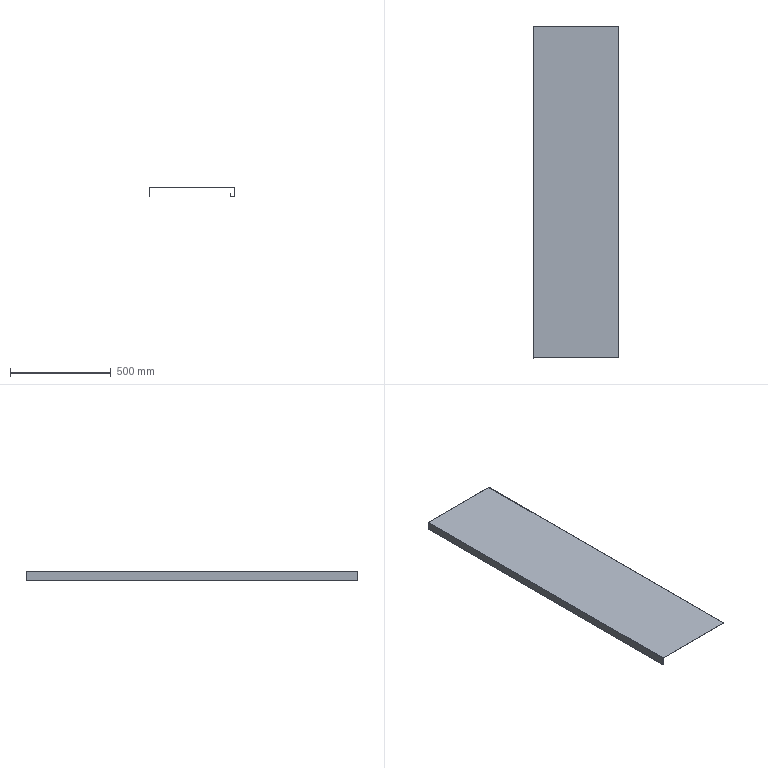Part | SolidWorks | features ExtruThin 1, ICE 1 | 1 solid | 15 faces | box 427 x 1649 x 42 mm | volume 892128 mm3 | plane 15
STEP:
#1=CARTESIAN_POINT('',(0.,0.,0.));
#2=VERTEX_POINT('',#1);
#3=CARTESIAN_POINT('',(426.,0.,0.));
#4=VERTEX_POINT('',#3);
#5=CARTESIAN_POINT('',(0.,0.,0.));
#6=DIRECTION('',(1.,0.,0.));
#7=VECTOR('',#6,1000.);
#8=LINE('',#5,#7);
#9=EDGE_CURVE('',#2,#4,#8,.T.);
#10=ORIENTED_EDGE('',*,*,#9,.T.);
#11=CARTESIAN_POINT('',(426.,0.,1.));
#12=VERTEX_POINT('',#11);
#13=CARTESIAN_POINT('',(426.,0.,0.));
#14=DIRECTION('',(0.,0.,-1.));
#15=VECTOR('',#14,1000.);
#16=LINE('',#13,#15);
#17=EDGE_CURVE('',#12,#4,#16,.T.);
#18=ORIENTED_EDGE('',*,*,#17,.F.);
#19=CARTESIAN_POINT('',(-1.,0.,1.));
#20=VERTEX_POINT('',#19);
#21=CARTESIAN_POINT('',(0.,0.,1.));
#22=DIRECTION('',(1.,0.,0.));
#23=VECTOR('',#22,1000.);
#24=LINE('',#21,#23);
#25=EDGE_CURVE('',#20,#12,#24,.T.);
#26=ORIENTED_EDGE('',*,*,#25,.F.);
#27=CARTESIAN_POINT('',(-1.,0.,-40.));
#28=VERTEX_POINT('',#27);
#29=CARTESIAN_POINT('',(-1.,0.,-40.));
#30=DIRECTION('',(0.,0.,1.));
#31=VECTOR('',#30,1000.);
#32=LINE('',#29,#31);
#33=EDGE_CURVE('',#28,#20,#32,.T.);
#34=ORIENTED_EDGE('',*,*,#33,.F.);
#35=CARTESIAN_POINT('',(0.,0.,-40.));
#36=VERTEX_POINT('',#35);
#37=CARTESIAN_POINT('',(-1.,0.,-40.));
#38=DIRECTION('',(1.,0.,0.));
#39=VECTOR('',#38,1000.);
#40=LINE('',#37,#39);
#41=EDGE_CURVE('',#28,#36,#40,.T.);
#42=ORIENTED_EDGE('',*,*,#41,.T.);
#43=CARTESIAN_POINT('',(0.,0.,-40.));
#44=DIRECTION('',(0.,0.,1.));
#45=VECTOR('',#44,1000.);
#46=LINE('',#43,#45);
#47=EDGE_CURVE('',#36,#2,#46,.T.);
#48=ORIENTED_EDGE('',*,*,#47,.T.);
#49=EDGE_LOOP('',(#10,#18,#26,#34,#42,#48));
#50=FACE_OUTER_BOUND('',#49,.T.);
#51=CARTESIAN_POINT('',(404.,0.,-25.));
#52=DIRECTION('',(0.,1.,0.));
#53=DIRECTION('',(1.,0.,0.));
#54=AXIS2_PLACEMENT_3D('',#51,#52,#53);
#55=PLANE('',#54);
#56=ADVANCED_FACE('',(#50),#55,.F.);
#57=CARTESIAN_POINT('',(404.,1649.,-41.));
#58=VERTEX_POINT('',#57);
#59=CARTESIAN_POINT('',(404.,64.,-41.));
#60=VERTEX_POINT('',#59);
#61=CARTESIAN_POINT('',(404.,1649.,-41.));
#62=DIRECTION('',(0.,-1.,0.));
#63=VECTOR('',#62,1000.);
#64=LINE('',#61,#63);
#65=EDGE_CURVE('',#58,#60,#64,.T.);
#66=ORIENTED_EDGE('',*,*,#65,.T.);
#67=CARTESIAN_POINT('',(404.,64.,-25.));
#68=VERTEX_POINT('',#67);
#69=CARTESIAN_POINT('',(404.,64.,67.676));
#70=DIRECTION('',(0.,0.,-1.));
#71=VECTOR('',#70,1000.);
#72=LINE('',#69,#71);
#73=EDGE_CURVE('',#68,#60,#72,.T.);
#74=ORIENTED_EDGE('',*,*,#73,.F.);
#75=CARTESIAN_POINT('',(404.,1649.,-25.));
#76=VERTEX_POINT('',#75);
#77=CARTESIAN_POINT('',(404.,1649.,-25.));
#78=DIRECTION('',(0.,-1.,0.));
#79=VECTOR('',#78,1000.);
#80=LINE('',#77,#79);
#81=EDGE_CURVE('',#76,#68,#80,.T.);
#82=ORIENTED_EDGE('',*,*,#81,.F.);
#83=CARTESIAN_POINT('',(404.,1649.,-40.));
#84=DIRECTION('',(0.,0.,1.));
#85=VECTOR('',#84,1000.);
#86=LINE('',#83,#85);
#87=EDGE_CURVE('',#58,#76,#86,.T.);
#88=ORIENTED_EDGE('',*,*,#87,.F.);
#89=EDGE_LOOP('',(#66,#74,#82,#88));
#90=FACE_OUTER_BOUND('',#89,.T.);
#91=CARTESIAN_POINT('',(404.,1649.,-40.));
#92=DIRECTION('',(1.,0.,0.));
#93=DIRECTION('',(0.,0.,-1.));
#94=AXIS2_PLACEMENT_3D('',#91,#92,#93);
#95=PLANE('',#94);
#96=ADVANCED_FACE('',(#90),#95,.F.);
#97=CARTESIAN_POINT('',(405.,64.,-25.));
#98=VERTEX_POINT('',#97);
#99=CARTESIAN_POINT('',(405.,64.,-25.));
#100=DIRECTION('',(-1.,0.,0.));
#101=VECTOR('',#100,1000.);
#102=LINE('',#99,#101);
#103=EDGE_CURVE('',#98,#68,#102,.T.);
#104=ORIENTED_EDGE('',*,*,#103,.F.);
#105=CARTESIAN_POINT('',(405.,1649.,-25.));
#106=VERTEX_POINT('',#105);
#107=CARTESIAN_POINT('',(405.,1649.,-25.));
#108=DIRECTION('',(0.,-1.,0.));
#109=VECTOR('',#108,1000.);
#110=LINE('',#107,#109);
#111=EDGE_CURVE('',#106,#98,#110,.T.);
#112=ORIENTED_EDGE('',*,*,#111,.F.);
#113=CARTESIAN_POINT('',(405.,1649.,-25.));
#114=DIRECTION('',(-1.,0.,0.));
#115=VECTOR('',#114,1000.);
#116=LINE('',#113,#115);
#117=EDGE_CURVE('',#106,#76,#116,.T.);
#118=ORIENTED_EDGE('',*,*,#117,.T.);
#119=ORIENTED_EDGE('',*,*,#81,.T.);
#120=EDGE_LOOP('',(#104,#112,#118,#119));
#121=FACE_OUTER_BOUND('',#120,.T.);
#122=CARTESIAN_POINT('',(405.,1649.,-25.));
#123=DIRECTION('',(0.,0.,1.));
#124=DIRECTION('',(1.,0.,0.));
#125=AXIS2_PLACEMENT_3D('',#122,#123,#124);
#126=PLANE('',#125);
#127=ADVANCED_FACE('',(#121),#126,.T.);
#128=CARTESIAN_POINT('',(405.,64.,-40.));
#129=VERTEX_POINT('',#128);
#130=CARTESIAN_POINT('',(405.,64.,-40.));
#131=DIRECTION('',(0.,0.,1.));
#132=VECTOR('',#131,1000.);
#133=LINE('',#130,#132);
#134=EDGE_CURVE('',#129,#98,#133,.T.);
#135=ORIENTED_EDGE('',*,*,#134,.F.);
#136=CARTESIAN_POINT('',(405.,1649.,-40.));
#137=VERTEX_POINT('',#136);
#138=CARTESIAN_POINT('',(405.,1649.,-40.));
#139=DIRECTION('',(0.,-1.,0.));
#140=VECTOR('',#139,1000.);
#141=LINE('',#138,#140);
#142=EDGE_CURVE('',#137,#129,#141,.T.);
#143=ORIENTED_EDGE('',*,*,#142,.F.);
#144=CARTESIAN_POINT('',(405.,1649.,-40.));
#145=DIRECTION('',(0.,0.,1.));
#146=VECTOR('',#145,1000.);
#147=LINE('',#144,#146);
#148=EDGE_CURVE('',#137,#106,#147,.T.);
#149=ORIENTED_EDGE('',*,*,#148,.T.);
#150=ORIENTED_EDGE('',*,*,#111,.T.);
#151=EDGE_LOOP('',(#135,#143,#149,#150));
#152=FACE_OUTER_BOUND('',#151,.T.);
#153=CARTESIAN_POINT('',(405.,1649.,-40.));
#154=DIRECTION('',(1.,0.,0.));
#155=DIRECTION('',(0.,0.,-1.));
#156=AXIS2_PLACEMENT_3D('',#153,#154,#155);
#157=PLANE('',#156);
#158=ADVANCED_FACE('',(#152),#157,.T.);
#159=CARTESIAN_POINT('',(425.,64.,-40.));
#160=VERTEX_POINT('',#159);
#161=CARTESIAN_POINT('',(425.,64.,-40.));
#162=DIRECTION('',(-1.,0.,0.));
#163=VECTOR('',#162,1000.);
#164=LINE('',#161,#163);
#165=EDGE_CURVE('',#160,#129,#164,.T.);
#166=ORIENTED_EDGE('',*,*,#165,.F.);
#167=CARTESIAN_POINT('',(425.,1649.,-40.));
#168=VERTEX_POINT('',#167);
#169=CARTESIAN_POINT('',(425.,1649.,-40.));
#170=DIRECTION('',(0.,-1.,0.));
#171=VECTOR('',#170,1000.);
#172=LINE('',#169,#171);
#173=EDGE_CURVE('',#168,#160,#172,.T.);
#174=ORIENTED_EDGE('',*,*,#173,.F.);
#175=CARTESIAN_POINT('',(425.,1649.,-40.));
#176=DIRECTION('',(-1.,0.,0.));
#177=VECTOR('',#176,1000.);
#178=LINE('',#175,#177);
#179=EDGE_CURVE('',#168,#137,#178,.T.);
#180=ORIENTED_EDGE('',*,*,#179,.T.);
#181=ORIENTED_EDGE('',*,*,#142,.T.);
#182=EDGE_LOOP('',(#166,#174,#180,#181));
#183=FACE_OUTER_BOUND('',#182,.T.);
#184=CARTESIAN_POINT('',(425.,1649.,-40.));
#185=DIRECTION('',(0.,0.,1.));
#186=DIRECTION('',(1.,0.,0.));
#187=AXIS2_PLACEMENT_3D('',#184,#185,#186);
#188=PLANE('',#187);
#189=ADVANCED_FACE('',(#183),#188,.T.);
#190=CARTESIAN_POINT('',(425.,64.,0.));
#191=VERTEX_POINT('',#190);
#192=CARTESIAN_POINT('',(425.,64.,0.));
#193=DIRECTION('',(0.,0.,-1.));
#194=VECTOR('',#193,1000.);
#195=LINE('',#192,#194);
#196=EDGE_CURVE('',#191,#160,#195,.T.);
#197=ORIENTED_EDGE('',*,*,#196,.F.);
#198=CARTESIAN_POINT('',(425.,1649.,0.));
#199=VERTEX_POINT('',#198);
#200=CARTESIAN_POINT('',(425.,1649.,0.));
#201=DIRECTION('',(0.,-1.,0.));
#202=VECTOR('',#201,1000.);
#203=LINE('',#200,#202);
#204=EDGE_CURVE('',#199,#191,#203,.T.);
#205=ORIENTED_EDGE('',*,*,#204,.F.);
#206=CARTESIAN_POINT('',(425.,1649.,0.));
#207=DIRECTION('',(0.,0.,-1.));
#208=VECTOR('',#207,1000.);
#209=LINE('',#206,#208);
#210=EDGE_CURVE('',#199,#168,#209,.T.);
#211=ORIENTED_EDGE('',*,*,#210,.T.);
#212=ORIENTED_EDGE('',*,*,#173,.T.);
#213=EDGE_LOOP('',(#197,#205,#211,#212));
#214=FACE_OUTER_BOUND('',#213,.T.);
#215=CARTESIAN_POINT('',(425.,1649.,0.));
#216=DIRECTION('',(-1.,0.,0.));
#217=DIRECTION('',(0.,0.,1.));
#218=AXIS2_PLACEMENT_3D('',#215,#216,#217);
#219=PLANE('',#218);
#220=ADVANCED_FACE('',(#214),#219,.T.);
#221=ORIENTED_EDGE('',*,*,#204,.T.);
#222=CARTESIAN_POINT('',(426.,64.,0.));
#223=VERTEX_POINT('',#222);
#224=CARTESIAN_POINT('',(426.,64.,0.));
#225=DIRECTION('',(-1.,0.,0.));
#226=VECTOR('',#225,1000.);
#227=LINE('',#224,#226);
#228=EDGE_CURVE('',#223,#191,#227,.T.);
#229=ORIENTED_EDGE('',*,*,#228,.F.);
#230=CARTESIAN_POINT('',(426.,0.,0.));
#231=DIRECTION('',(0.,1.,0.));
#232=VECTOR('',#231,1000.);
#233=LINE('',#230,#232);
#234=EDGE_CURVE('',#4,#223,#233,.T.);
#235=ORIENTED_EDGE('',*,*,#234,.F.);
#236=ORIENTED_EDGE('',*,*,#9,.F.);
#237=CARTESIAN_POINT('',(0.,1649.,0.));
#238=VERTEX_POINT('',#237);
#239=CARTESIAN_POINT('',(0.,1649.,0.));
#240=DIRECTION('',(0.,-1.,0.));
#241=VECTOR('',#240,1000.);
#242=LINE('',#239,#241);
#243=EDGE_CURVE('',#238,#2,#242,.T.);
#244=ORIENTED_EDGE('',*,*,#243,.F.);
#245=CARTESIAN_POINT('',(0.,1649.,0.));
#246=DIRECTION('',(1.,0.,0.));
#247=VECTOR('',#246,1000.);
#248=LINE('',#245,#247);
#249=EDGE_CURVE('',#238,#199,#248,.T.);
#250=ORIENTED_EDGE('',*,*,#249,.T.);
#251=EDGE_LOOP('',(#221,#229,#235,#236,#244,#250));
#252=FACE_OUTER_BOUND('',#251,.T.);
#253=CARTESIAN_POINT('',(0.,1649.,0.));
#254=DIRECTION('',(0.,0.,-1.));
#255=DIRECTION('',(-1.,0.,0.));
#256=AXIS2_PLACEMENT_3D('',#253,#254,#255);
#257=PLANE('',#256);
#258=ADVANCED_FACE('',(#252),#257,.T.);
#259=ORIENTED_EDGE('',*,*,#47,.F.);
#260=CARTESIAN_POINT('',(0.,1649.,-40.));
#261=VERTEX_POINT('',#260);
#262=CARTESIAN_POINT('',(0.,1649.,-40.));
#263=DIRECTION('',(0.,-1.,0.));
#264=VECTOR('',#263,1000.);
#265=LINE('',#262,#264);
#266=EDGE_CURVE('',#261,#36,#265,.T.);
#267=ORIENTED_EDGE('',*,*,#266,.F.);
#268=CARTESIAN_POINT('',(0.,1649.,-40.));
#269=DIRECTION('',(0.,0.,1.));
#270=VECTOR('',#269,1000.);
#271=LINE('',#268,#270);
#272=EDGE_CURVE('',#261,#238,#271,.T.);
#273=ORIENTED_EDGE('',*,*,#272,.T.);
#274=ORIENTED_EDGE('',*,*,#243,.T.);
#275=EDGE_LOOP('',(#259,#267,#273,#274));
#276=FACE_OUTER_BOUND('',#275,.T.);
#277=CARTESIAN_POINT('',(0.,1649.,-40.));
#278=DIRECTION('',(1.,0.,0.));
#279=DIRECTION('',(0.,0.,-1.));
#280=AXIS2_PLACEMENT_3D('',#277,#278,#279);
#281=PLANE('',#280);
#282=ADVANCED_FACE('',(#276),#281,.T.);
#283=ORIENTED_EDGE('',*,*,#41,.F.);
#284=CARTESIAN_POINT('',(-1.,1649.,-40.));
#285=VERTEX_POINT('',#284);
#286=CARTESIAN_POINT('',(-1.,1649.,-40.));
#287=DIRECTION('',(0.,-1.,0.));
#288=VECTOR('',#287,1000.);
#289=LINE('',#286,#288);
#290=EDGE_CURVE('',#285,#28,#289,.T.);
#291=ORIENTED_EDGE('',*,*,#290,.F.);
#292=CARTESIAN_POINT('',(-1.,1649.,-40.));
#293=DIRECTION('',(1.,0.,0.));
#294=VECTOR('',#293,1000.);
#295=LINE('',#292,#294);
#296=EDGE_CURVE('',#285,#261,#295,.T.);
#297=ORIENTED_EDGE('',*,*,#296,.T.);
#298=ORIENTED_EDGE('',*,*,#266,.T.);
#299=EDGE_LOOP('',(#283,#291,#297,#298));
#300=FACE_OUTER_BOUND('',#299,.T.);
#301=CARTESIAN_POINT('',(-1.,1649.,-40.));
#302=DIRECTION('',(0.,0.,-1.));
#303=DIRECTION('',(-1.,0.,0.));
#304=AXIS2_PLACEMENT_3D('',#301,#302,#303);
#305=PLANE('',#304);
#306=ADVANCED_FACE('',(#300),#305,.T.);
#307=ORIENTED_EDGE('',*,*,#33,.T.);
#308=CARTESIAN_POINT('',(-1.,1649.,1.));
#309=VERTEX_POINT('',#308);
#310=CARTESIAN_POINT('',(-1.,1649.,1.));
#311=DIRECTION('',(0.,-1.,0.));
#312=VECTOR('',#311,1000.);
#313=LINE('',#310,#312);
#314=EDGE_CURVE('',#309,#20,#313,.T.);
#315=ORIENTED_EDGE('',*,*,#314,.F.);
#316=CARTESIAN_POINT('',(-1.,1649.,-40.));
#317=DIRECTION('',(0.,0.,1.));
#318=VECTOR('',#317,1000.);
#319=LINE('',#316,#318);
#320=EDGE_CURVE('',#285,#309,#319,.T.);
#321=ORIENTED_EDGE('',*,*,#320,.F.);
#322=ORIENTED_EDGE('',*,*,#290,.T.);
#323=EDGE_LOOP('',(#307,#315,#321,#322));
#324=FACE_OUTER_BOUND('',#323,.T.);
#325=CARTESIAN_POINT('',(-1.,1649.,-40.));
#326=DIRECTION('',(1.,0.,0.));
#327=DIRECTION('',(0.,0.,-1.));
#328=AXIS2_PLACEMENT_3D('',#325,#326,#327);
#329=PLANE('',#328);
#330=ADVANCED_FACE('',(#324),#329,.F.);
#331=ORIENTED_EDGE('',*,*,#25,.T.);
#332=CARTESIAN_POINT('',(426.,1649.,1.));
#333=VERTEX_POINT('',#332);
#334=CARTESIAN_POINT('',(426.,1649.,1.));
#335=DIRECTION('',(0.,-1.,0.));
#336=VECTOR('',#335,1000.);
#337=LINE('',#334,#336);
#338=EDGE_CURVE('',#333,#12,#337,.T.);
#339=ORIENTED_EDGE('',*,*,#338,.F.);
#340=CARTESIAN_POINT('',(0.,1649.,1.));
#341=DIRECTION('',(1.,0.,0.));
#342=VECTOR('',#341,1000.);
#343=LINE('',#340,#342);
#344=EDGE_CURVE('',#309,#333,#343,.T.);
#345=ORIENTED_EDGE('',*,*,#344,.F.);
#346=ORIENTED_EDGE('',*,*,#314,.T.);
#347=EDGE_LOOP('',(#331,#339,#345,#346));
#348=FACE_OUTER_BOUND('',#347,.T.);
#349=CARTESIAN_POINT('',(0.,1649.,1.));
#350=DIRECTION('',(0.,0.,-1.));
#351=DIRECTION('',(-1.,0.,0.));
#352=AXIS2_PLACEMENT_3D('',#349,#350,#351);
#353=PLANE('',#352);
#354=ADVANCED_FACE('',(#348),#353,.F.);
#355=ORIENTED_EDGE('',*,*,#234,.T.);
#356=CARTESIAN_POINT('',(426.,64.,-41.));
#357=VERTEX_POINT('',#356);
#358=CARTESIAN_POINT('',(426.,64.,67.676));
#359=DIRECTION('',(0.,0.,-1.));
#360=VECTOR('',#359,1000.);
#361=LINE('',#358,#360);
#362=EDGE_CURVE('',#223,#357,#361,.T.);
#363=ORIENTED_EDGE('',*,*,#362,.T.);
#364=CARTESIAN_POINT('',(426.,1649.,-41.));
#365=VERTEX_POINT('',#364);
#366=CARTESIAN_POINT('',(426.,1649.,-41.));
#367=DIRECTION('',(0.,-1.,0.));
#368=VECTOR('',#367,1000.);
#369=LINE('',#366,#368);
#370=EDGE_CURVE('',#365,#357,#369,.T.);
#371=ORIENTED_EDGE('',*,*,#370,.F.);
#372=CARTESIAN_POINT('',(426.,1649.,0.));
#373=DIRECTION('',(0.,0.,-1.));
#374=VECTOR('',#373,1000.);
#375=LINE('',#372,#374);
#376=EDGE_CURVE('',#333,#365,#375,.T.);
#377=ORIENTED_EDGE('',*,*,#376,.F.);
#378=ORIENTED_EDGE('',*,*,#338,.T.);
#379=ORIENTED_EDGE('',*,*,#17,.T.);
#380=EDGE_LOOP('',(#355,#363,#371,#377,#378,#379));
#381=FACE_OUTER_BOUND('',#380,.T.);
#382=CARTESIAN_POINT('',(426.,1649.,0.));
#383=DIRECTION('',(-1.,0.,0.));
#384=DIRECTION('',(0.,0.,1.));
#385=AXIS2_PLACEMENT_3D('',#382,#383,#384);
#386=PLANE('',#385);
#387=ADVANCED_FACE('',(#381),#386,.F.);
#388=ORIENTED_EDGE('',*,*,#370,.T.);
#389=CARTESIAN_POINT('',(426.,64.,-41.));
#390=DIRECTION('',(1.,0.,0.));
#391=VECTOR('',#390,1000.);
#392=LINE('',#389,#391);
#393=EDGE_CURVE('',#60,#357,#392,.T.);
#394=ORIENTED_EDGE('',*,*,#393,.F.);
#395=ORIENTED_EDGE('',*,*,#65,.F.);
#396=CARTESIAN_POINT('',(425.,1649.,-41.));
#397=DIRECTION('',(-1.,0.,0.));
#398=VECTOR('',#397,1000.);
#399=LINE('',#396,#398);
#400=EDGE_CURVE('',#365,#58,#399,.T.);
#401=ORIENTED_EDGE('',*,*,#400,.F.);
#402=EDGE_LOOP('',(#388,#394,#395,#401));
#403=FACE_OUTER_BOUND('',#402,.T.);
#404=CARTESIAN_POINT('',(425.,1649.,-41.));
#405=DIRECTION('',(0.,0.,1.));
#406=DIRECTION('',(1.,0.,0.));
#407=AXIS2_PLACEMENT_3D('',#404,#405,#406);
#408=PLANE('',#407);
#409=ADVANCED_FACE('',(#403),#408,.F.);
#410=ORIENTED_EDGE('',*,*,#87,.T.);
#411=ORIENTED_EDGE('',*,*,#117,.F.);
#412=ORIENTED_EDGE('',*,*,#148,.F.);
#413=ORIENTED_EDGE('',*,*,#179,.F.);
#414=ORIENTED_EDGE('',*,*,#210,.F.);
#415=ORIENTED_EDGE('',*,*,#249,.F.);
#416=ORIENTED_EDGE('',*,*,#272,.F.);
#417=ORIENTED_EDGE('',*,*,#296,.F.);
#418=ORIENTED_EDGE('',*,*,#320,.T.);
#419=ORIENTED_EDGE('',*,*,#344,.T.);
#420=ORIENTED_EDGE('',*,*,#376,.T.);
#421=ORIENTED_EDGE('',*,*,#400,.T.);
#422=EDGE_LOOP('',(#410,#411,#412,#413,#414,#415,#416,#417,#418,#419,#420,#421));
#423=FACE_OUTER_BOUND('',#422,.T.);
#424=CARTESIAN_POINT('',(404.,1649.,-25.));
#425=DIRECTION('',(0.,1.,0.));
#426=DIRECTION('',(1.,0.,0.));
#427=AXIS2_PLACEMENT_3D('',#424,#425,#426);
#428=PLANE('',#427);
#429=ADVANCED_FACE('',(#423),#428,.T.);
#430=ORIENTED_EDGE('',*,*,#103,.T.);
#431=ORIENTED_EDGE('',*,*,#73,.T.);
#432=ORIENTED_EDGE('',*,*,#393,.T.);
#433=ORIENTED_EDGE('',*,*,#362,.F.);
#434=ORIENTED_EDGE('',*,*,#228,.T.);
#435=ORIENTED_EDGE('',*,*,#196,.T.);
#436=ORIENTED_EDGE('',*,*,#165,.T.);
#437=ORIENTED_EDGE('',*,*,#134,.T.);
#438=EDGE_LOOP('',(#430,#431,#432,#433,#434,#435,#436,#437));
#439=FACE_OUTER_BOUND('',#438,.T.);
#440=CARTESIAN_POINT('',(426.,64.,67.676));
#441=DIRECTION('',(0.,1.,0.));
#442=DIRECTION('',(0.,0.,1.));
#443=AXIS2_PLACEMENT_3D('',#440,#441,#442);
#444=PLANE('',#443);
#445=ADVANCED_FACE('',(#439),#444,.F.);
#446=CLOSED_SHELL('',(#56,#96,#127,#158,#189,#220,#258,#282,#306,#330,#354,#387,#409,#429,#445));
#447=MANIFOLD_SOLID_BREP('',#446);
#448=CARTESIAN_POINT('',(0.,0.,0.));
#449=DIRECTION('',(0.,0.,1.));
#450=DIRECTION('',(1.,0.,0.));
#451=AXIS2_PLACEMENT_3D('',#448,#449,#450);
#452=(LENGTH_UNIT()NAMED_UNIT(*)SI_UNIT(.MILLI.,.METRE.));
#453=UNCERTAINTY_MEASURE_WITH_UNIT(LENGTH_MEASURE(0.00001),#452,'','');
#454=(NAMED_UNIT(*)PLANE_ANGLE_UNIT()SI_UNIT($,.RADIAN.));
#455=(NAMED_UNIT(*)SI_UNIT($,.STERADIAN.)SOLID_ANGLE_UNIT());
#456=(GEOMETRIC_REPRESENTATION_CONTEXT(3)GLOBAL_UNCERTAINTY_ASSIGNED_CONTEXT((#453))GLOBAL_UNIT_ASSIGNED_CONTEXT((#452,#454,#455))REPRESENTATION_CONTEXT('',''));
#457=ADVANCED_BREP_SHAPE_REPRESENTATION('',(#447,#451),#456);